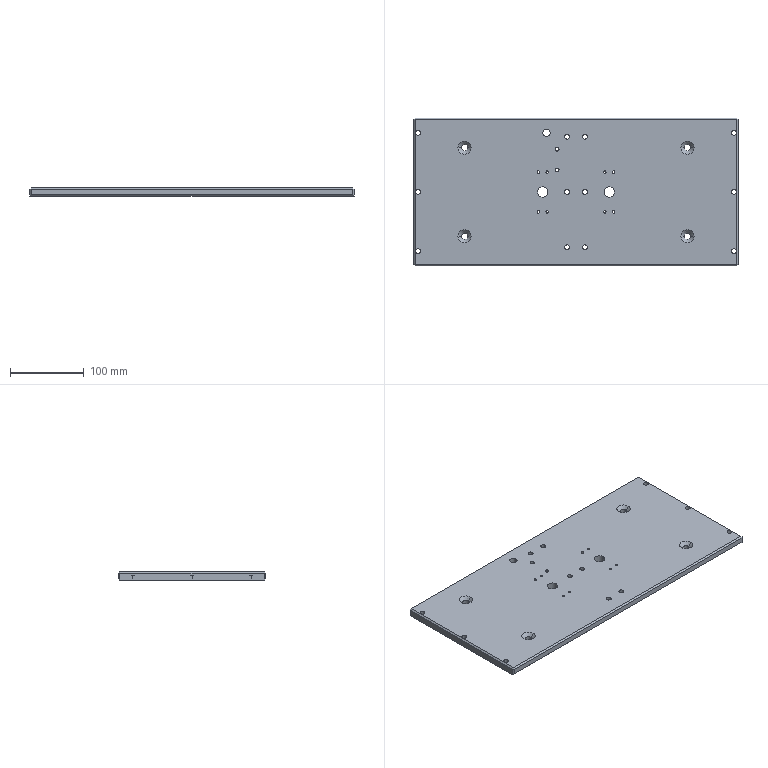Part | STEP file | Rotor mis-part check fixture-base plate | 1 solid | 122 faces | box 440 x 200 x 11 mm | volume 944706 mm3 | cylinder 82 | plane 32 | cone 8 | commonest cylinder face diameters 6.6 x24 11 x24 3.3 x16 9 x8 5 x4 14 x4